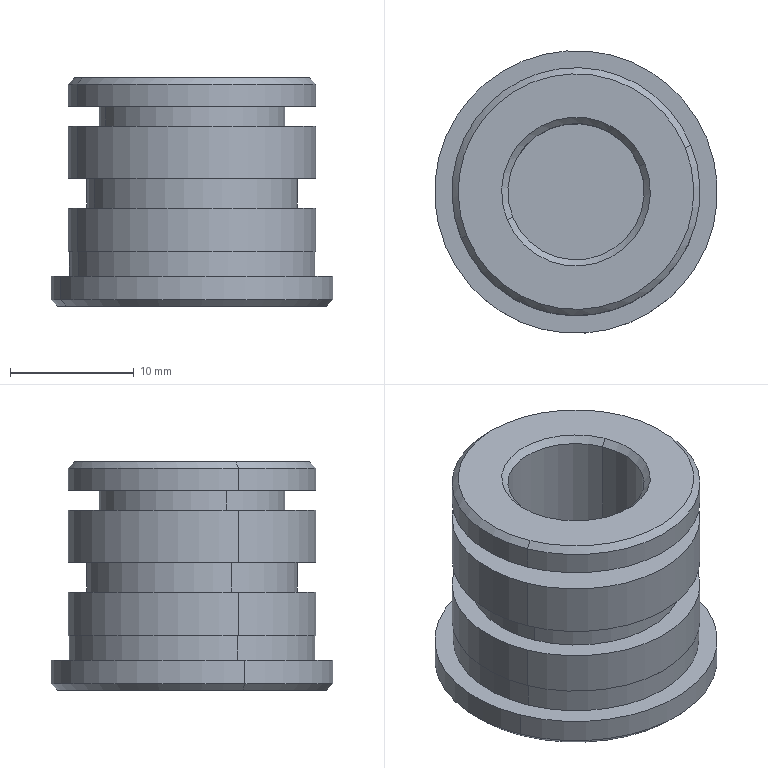Part | SolidWorks | features BaseBody 1 | 1 solid | 34 faces | box 22.8 x 22.8 x 18.4 mm | volume 3781 mm3 | cylinder 18 | plane 10 | cone 6 | commonest cylinder face diameters 20 x6 15 x4 11 x2 17 x2 19.8 x2 22.8 x2
STEP:
#1=CARTESIAN_POINT('',(372.994,98.417,-49.5));
#2=VERTEX_POINT('',#1);
#3=CARTESIAN_POINT('',(393.206,106.583,-49.5));
#4=VERTEX_POINT('',#3);
#5=CARTESIAN_POINT('',(383.1,102.5,-49.5));
#6=DIRECTION('',(0.,0.,1.));
#7=DIRECTION('',(-0.9272,-0.3746,0.));
#8=AXIS2_PLACEMENT_3D('',#5,#6,#7);
#9=CIRCLE('',#8,10.9);
#10=EDGE_CURVE('',#2,#4,#9,.T.);
#11=ORIENTED_EDGE('',*,*,#10,.T.);
#12=CARTESIAN_POINT('',(393.67,106.77,-49.));
#13=VERTEX_POINT('',#12);
#14=CARTESIAN_POINT('',(393.67,106.77,-49.));
#15=DIRECTION('',(0.6556,0.2649,0.7071));
#16=VECTOR('',#15,1000.);
#17=LINE('',#14,#16);
#18=EDGE_CURVE('',#4,#13,#17,.T.);
#19=ORIENTED_EDGE('',*,*,#18,.T.);
#20=CARTESIAN_POINT('',(372.53,98.23,-49.));
#21=VERTEX_POINT('',#20);
#22=CARTESIAN_POINT('',(383.1,102.5,-49.));
#23=DIRECTION('',(0.,0.,1.));
#24=DIRECTION('',(-0.9272,-0.3746,0.));
#25=AXIS2_PLACEMENT_3D('',#22,#23,#24);
#26=CIRCLE('',#25,11.4);
#27=EDGE_CURVE('',#21,#13,#26,.T.);
#28=ORIENTED_EDGE('',*,*,#27,.F.);
#29=CARTESIAN_POINT('',(372.53,98.23,-49.));
#30=DIRECTION('',(-0.6556,-0.2649,0.7071));
#31=VECTOR('',#30,1000.);
#32=LINE('',#29,#31);
#33=EDGE_CURVE('',#2,#21,#32,.T.);
#34=ORIENTED_EDGE('',*,*,#33,.F.);
#35=EDGE_LOOP('',(#11,#19,#28,#34));
#36=FACE_OUTER_BOUND('',#35,.T.);
#37=CARTESIAN_POINT('',(383.1,102.5,-49.));
#38=DIRECTION('',(0.,0.,1.));
#39=DIRECTION('',(-0.9272,-0.3746,0.));
#40=AXIS2_PLACEMENT_3D('',#37,#38,#39);
#41=CONICAL_SURFACE('',#40,11.4,0.7854);
#42=ADVANCED_FACE('',(#36),#41,.T.);
#43=ORIENTED_EDGE('',*,*,#27,.T.);
#44=CARTESIAN_POINT('',(393.67,106.77,-47.1));
#45=VERTEX_POINT('',#44);
#46=CARTESIAN_POINT('',(393.67,106.77,-25.779));
#47=DIRECTION('',(0.,0.,1.));
#48=VECTOR('',#47,1000.);
#49=LINE('',#46,#48);
#50=EDGE_CURVE('',#13,#45,#49,.T.);
#51=ORIENTED_EDGE('',*,*,#50,.T.);
#52=CARTESIAN_POINT('',(372.53,98.23,-47.1));
#53=VERTEX_POINT('',#52);
#54=CARTESIAN_POINT('',(383.1,102.5,-47.1));
#55=DIRECTION('',(0.,0.,1.));
#56=DIRECTION('',(-0.9272,-0.3746,0.));
#57=AXIS2_PLACEMENT_3D('',#54,#55,#56);
#58=CIRCLE('',#57,11.4);
#59=EDGE_CURVE('',#53,#45,#58,.T.);
#60=ORIENTED_EDGE('',*,*,#59,.F.);
#61=CARTESIAN_POINT('',(372.53,98.23,-25.779));
#62=DIRECTION('',(0.,0.,1.));
#63=VECTOR('',#62,1000.);
#64=LINE('',#61,#63);
#65=EDGE_CURVE('',#21,#53,#64,.T.);
#66=ORIENTED_EDGE('',*,*,#65,.F.);
#67=EDGE_LOOP('',(#43,#51,#60,#66));
#68=FACE_OUTER_BOUND('',#67,.T.);
#69=CARTESIAN_POINT('',(383.1,102.5,-25.779));
#70=DIRECTION('',(0.,0.,1.));
#71=DIRECTION('',(-0.9272,-0.3746,0.));
#72=AXIS2_PLACEMENT_3D('',#69,#70,#71);
#73=CYLINDRICAL_SURFACE('',#72,11.4);
#74=ADVANCED_FACE('',(#68),#73,.T.);
#75=CARTESIAN_POINT('',(373.921,98.792,-47.1));
#76=VERTEX_POINT('',#75);
#77=CARTESIAN_POINT('',(392.279,106.208,-47.1));
#78=VERTEX_POINT('',#77);
#79=CARTESIAN_POINT('',(383.1,102.5,-47.1));
#80=DIRECTION('',(0.,0.,1.));
#81=DIRECTION('',(-0.9272,-0.3746,0.));
#82=AXIS2_PLACEMENT_3D('',#79,#80,#81);
#83=CIRCLE('',#82,9.9);
#84=EDGE_CURVE('',#76,#78,#83,.T.);
#85=ORIENTED_EDGE('',*,*,#84,.T.);
#86=CARTESIAN_POINT('',(392.279,106.208,-45.1));
#87=VERTEX_POINT('',#86);
#88=CARTESIAN_POINT('',(392.279,106.208,-25.779));
#89=DIRECTION('',(0.,0.,1.));
#90=VECTOR('',#89,1000.);
#91=LINE('',#88,#90);
#92=EDGE_CURVE('',#78,#87,#91,.T.);
#93=ORIENTED_EDGE('',*,*,#92,.T.);
#94=CARTESIAN_POINT('',(373.921,98.792,-45.1));
#95=VERTEX_POINT('',#94);
#96=CARTESIAN_POINT('',(383.1,102.5,-45.1));
#97=DIRECTION('',(0.,0.,1.));
#98=DIRECTION('',(-0.9272,-0.3746,0.));
#99=AXIS2_PLACEMENT_3D('',#96,#97,#98);
#100=CIRCLE('',#99,9.9);
#101=EDGE_CURVE('',#95,#87,#100,.T.);
#102=ORIENTED_EDGE('',*,*,#101,.F.);
#103=CARTESIAN_POINT('',(373.921,98.792,-25.779));
#104=DIRECTION('',(0.,0.,1.));
#105=VECTOR('',#104,1000.);
#106=LINE('',#103,#105);
#107=EDGE_CURVE('',#76,#95,#106,.T.);
#108=ORIENTED_EDGE('',*,*,#107,.F.);
#109=EDGE_LOOP('',(#85,#93,#102,#108));
#110=FACE_OUTER_BOUND('',#109,.T.);
#111=CARTESIAN_POINT('',(383.1,102.5,-25.779));
#112=DIRECTION('',(0.,0.,1.));
#113=DIRECTION('',(-0.9272,-0.3746,0.));
#114=AXIS2_PLACEMENT_3D('',#111,#112,#113);
#115=CYLINDRICAL_SURFACE('',#114,9.9);
#116=ADVANCED_FACE('',(#110),#115,.T.);
#117=CARTESIAN_POINT('',(373.828,98.754,-45.1));
#118=VERTEX_POINT('',#117);
#119=CARTESIAN_POINT('',(392.372,106.246,-45.1));
#120=VERTEX_POINT('',#119);
#121=CARTESIAN_POINT('',(383.1,102.5,-45.1));
#122=DIRECTION('',(0.,0.,1.));
#123=DIRECTION('',(-0.9272,-0.3746,0.));
#124=AXIS2_PLACEMENT_3D('',#121,#122,#123);
#125=CIRCLE('',#124,10.);
#126=EDGE_CURVE('',#118,#120,#125,.T.);
#127=ORIENTED_EDGE('',*,*,#126,.T.);
#128=CARTESIAN_POINT('',(392.372,106.246,-41.6));
#129=VERTEX_POINT('',#128);
#130=CARTESIAN_POINT('',(392.372,106.246,-25.779));
#131=DIRECTION('',(0.,0.,1.));
#132=VECTOR('',#131,1000.);
#133=LINE('',#130,#132);
#134=EDGE_CURVE('',#120,#129,#133,.T.);
#135=ORIENTED_EDGE('',*,*,#134,.T.);
#136=CARTESIAN_POINT('',(373.828,98.754,-41.6));
#137=VERTEX_POINT('',#136);
#138=CARTESIAN_POINT('',(383.1,102.5,-41.6));
#139=DIRECTION('',(0.,0.,1.));
#140=DIRECTION('',(-0.9272,-0.3746,0.));
#141=AXIS2_PLACEMENT_3D('',#138,#139,#140);
#142=CIRCLE('',#141,10.);
#143=EDGE_CURVE('',#137,#129,#142,.T.);
#144=ORIENTED_EDGE('',*,*,#143,.F.);
#145=CARTESIAN_POINT('',(373.828,98.754,-25.779));
#146=DIRECTION('',(0.,0.,1.));
#147=VECTOR('',#146,1000.);
#148=LINE('',#145,#147);
#149=EDGE_CURVE('',#118,#137,#148,.T.);
#150=ORIENTED_EDGE('',*,*,#149,.F.);
#151=EDGE_LOOP('',(#127,#135,#144,#150));
#152=FACE_OUTER_BOUND('',#151,.T.);
#153=CARTESIAN_POINT('',(383.1,102.5,-25.779));
#154=DIRECTION('',(0.,0.,1.));
#155=DIRECTION('',(-0.9272,-0.3746,0.));
#156=AXIS2_PLACEMENT_3D('',#153,#154,#155);
#157=CYLINDRICAL_SURFACE('',#156,10.);
#158=ADVANCED_FACE('',(#152),#157,.T.);
#159=CARTESIAN_POINT('',(375.219,99.316,-41.6));
#160=VERTEX_POINT('',#159);
#161=CARTESIAN_POINT('',(390.981,105.684,-41.6));
#162=VERTEX_POINT('',#161);
#163=CARTESIAN_POINT('',(383.1,102.5,-41.6));
#164=DIRECTION('',(0.,0.,1.));
#165=DIRECTION('',(-0.9272,-0.3746,0.));
#166=AXIS2_PLACEMENT_3D('',#163,#164,#165);
#167=CIRCLE('',#166,8.5);
#168=EDGE_CURVE('',#160,#162,#167,.T.);
#169=ORIENTED_EDGE('',*,*,#168,.T.);
#170=CARTESIAN_POINT('',(390.981,105.684,-39.2));
#171=VERTEX_POINT('',#170);
#172=CARTESIAN_POINT('',(390.981,105.684,-25.779));
#173=DIRECTION('',(0.,0.,1.));
#174=VECTOR('',#173,1000.);
#175=LINE('',#172,#174);
#176=EDGE_CURVE('',#162,#171,#175,.T.);
#177=ORIENTED_EDGE('',*,*,#176,.T.);
#178=CARTESIAN_POINT('',(375.219,99.316,-39.2));
#179=VERTEX_POINT('',#178);
#180=CARTESIAN_POINT('',(383.1,102.5,-39.2));
#181=DIRECTION('',(0.,0.,1.));
#182=DIRECTION('',(-0.9272,-0.3746,0.));
#183=AXIS2_PLACEMENT_3D('',#180,#181,#182);
#184=CIRCLE('',#183,8.5);
#185=EDGE_CURVE('',#179,#171,#184,.T.);
#186=ORIENTED_EDGE('',*,*,#185,.F.);
#187=CARTESIAN_POINT('',(375.219,99.316,-25.779));
#188=DIRECTION('',(0.,0.,1.));
#189=VECTOR('',#188,1000.);
#190=LINE('',#187,#189);
#191=EDGE_CURVE('',#160,#179,#190,.T.);
#192=ORIENTED_EDGE('',*,*,#191,.F.);
#193=EDGE_LOOP('',(#169,#177,#186,#192));
#194=FACE_OUTER_BOUND('',#193,.T.);
#195=CARTESIAN_POINT('',(383.1,102.5,-25.779));
#196=DIRECTION('',(0.,0.,1.));
#197=DIRECTION('',(-0.9272,-0.3746,0.));
#198=AXIS2_PLACEMENT_3D('',#195,#196,#197);
#199=CYLINDRICAL_SURFACE('',#198,8.5);
#200=ADVANCED_FACE('',(#194),#199,.T.);
#201=CARTESIAN_POINT('',(373.828,98.754,-39.2));
#202=VERTEX_POINT('',#201);
#203=CARTESIAN_POINT('',(392.372,106.246,-39.2));
#204=VERTEX_POINT('',#203);
#205=CARTESIAN_POINT('',(383.1,102.5,-39.2));
#206=DIRECTION('',(0.,0.,1.));
#207=DIRECTION('',(-0.9272,-0.3746,0.));
#208=AXIS2_PLACEMENT_3D('',#205,#206,#207);
#209=CIRCLE('',#208,10.);
#210=EDGE_CURVE('',#202,#204,#209,.T.);
#211=ORIENTED_EDGE('',*,*,#210,.T.);
#212=CARTESIAN_POINT('',(392.372,106.246,-35.));
#213=VERTEX_POINT('',#212);
#214=CARTESIAN_POINT('',(392.372,106.246,-25.779));
#215=DIRECTION('',(0.,0.,1.));
#216=VECTOR('',#215,1000.);
#217=LINE('',#214,#216);
#218=EDGE_CURVE('',#204,#213,#217,.T.);
#219=ORIENTED_EDGE('',*,*,#218,.T.);
#220=CARTESIAN_POINT('',(373.828,98.754,-35.));
#221=VERTEX_POINT('',#220);
#222=CARTESIAN_POINT('',(383.1,102.5,-35.));
#223=DIRECTION('',(0.,0.,1.));
#224=DIRECTION('',(-0.9272,-0.3746,0.));
#225=AXIS2_PLACEMENT_3D('',#222,#223,#224);
#226=CIRCLE('',#225,10.);
#227=EDGE_CURVE('',#221,#213,#226,.T.);
#228=ORIENTED_EDGE('',*,*,#227,.F.);
#229=CARTESIAN_POINT('',(373.828,98.754,-25.779));
#230=DIRECTION('',(0.,0.,1.));
#231=VECTOR('',#230,1000.);
#232=LINE('',#229,#231);
#233=EDGE_CURVE('',#202,#221,#232,.T.);
#234=ORIENTED_EDGE('',*,*,#233,.F.);
#235=EDGE_LOOP('',(#211,#219,#228,#234));
#236=FACE_OUTER_BOUND('',#235,.T.);
#237=CARTESIAN_POINT('',(383.1,102.5,-25.779));
#238=DIRECTION('',(0.,0.,1.));
#239=DIRECTION('',(-0.9272,-0.3746,0.));
#240=AXIS2_PLACEMENT_3D('',#237,#238,#239);
#241=CYLINDRICAL_SURFACE('',#240,10.);
#242=ADVANCED_FACE('',(#236),#241,.T.);
#243=CARTESIAN_POINT('',(376.146,99.691,-35.));
#244=VERTEX_POINT('',#243);
#245=CARTESIAN_POINT('',(390.054,105.309,-35.));
#246=VERTEX_POINT('',#245);
#247=CARTESIAN_POINT('',(383.1,102.5,-35.));
#248=DIRECTION('',(0.,0.,1.));
#249=DIRECTION('',(-0.9272,-0.3746,0.));
#250=AXIS2_PLACEMENT_3D('',#247,#248,#249);
#251=CIRCLE('',#250,7.5);
#252=EDGE_CURVE('',#244,#246,#251,.T.);
#253=ORIENTED_EDGE('',*,*,#252,.T.);
#254=CARTESIAN_POINT('',(390.054,105.309,-33.4));
#255=VERTEX_POINT('',#254);
#256=CARTESIAN_POINT('',(390.054,105.309,-25.779));
#257=DIRECTION('',(0.,0.,1.));
#258=VECTOR('',#257,1000.);
#259=LINE('',#256,#258);
#260=EDGE_CURVE('',#246,#255,#259,.T.);
#261=ORIENTED_EDGE('',*,*,#260,.T.);
#262=CARTESIAN_POINT('',(376.146,99.691,-33.4));
#263=VERTEX_POINT('',#262);
#264=CARTESIAN_POINT('',(383.1,102.5,-33.4));
#265=DIRECTION('',(0.,0.,1.));
#266=DIRECTION('',(-0.9272,-0.3746,0.));
#267=AXIS2_PLACEMENT_3D('',#264,#265,#266);
#268=CIRCLE('',#267,7.5);
#269=EDGE_CURVE('',#263,#255,#268,.T.);
#270=ORIENTED_EDGE('',*,*,#269,.F.);
#271=CARTESIAN_POINT('',(376.146,99.691,-25.779));
#272=DIRECTION('',(0.,0.,1.));
#273=VECTOR('',#272,1000.);
#274=LINE('',#271,#273);
#275=EDGE_CURVE('',#244,#263,#274,.T.);
#276=ORIENTED_EDGE('',*,*,#275,.F.);
#277=EDGE_LOOP('',(#253,#261,#270,#276));
#278=FACE_OUTER_BOUND('',#277,.T.);
#279=CARTESIAN_POINT('',(383.1,102.5,-25.779));
#280=DIRECTION('',(0.,0.,1.));
#281=DIRECTION('',(-0.9272,-0.3746,0.));
#282=AXIS2_PLACEMENT_3D('',#279,#280,#281);
#283=CYLINDRICAL_SURFACE('',#282,7.5);
#284=ADVANCED_FACE('',(#278),#283,.T.);
#285=CARTESIAN_POINT('',(373.828,98.754,-33.4));
#286=VERTEX_POINT('',#285);
#287=CARTESIAN_POINT('',(392.372,106.246,-33.4));
#288=VERTEX_POINT('',#287);
#289=CARTESIAN_POINT('',(383.1,102.5,-33.4));
#290=DIRECTION('',(0.,0.,1.));
#291=DIRECTION('',(-0.9272,-0.3746,0.));
#292=AXIS2_PLACEMENT_3D('',#289,#290,#291);
#293=CIRCLE('',#292,10.);
#294=EDGE_CURVE('',#286,#288,#293,.T.);
#295=ORIENTED_EDGE('',*,*,#294,.T.);
#296=CARTESIAN_POINT('',(392.372,106.246,-31.6));
#297=VERTEX_POINT('',#296);
#298=CARTESIAN_POINT('',(392.372,106.246,-25.779));
#299=DIRECTION('',(0.,0.,1.));
#300=VECTOR('',#299,1000.);
#301=LINE('',#298,#300);
#302=EDGE_CURVE('',#288,#297,#301,.T.);
#303=ORIENTED_EDGE('',*,*,#302,.T.);
#304=CARTESIAN_POINT('',(373.828,98.754,-31.6));
#305=VERTEX_POINT('',#304);
#306=CARTESIAN_POINT('',(383.1,102.5,-31.6));
#307=DIRECTION('',(0.,0.,1.));
#308=DIRECTION('',(-0.9272,-0.3746,0.));
#309=AXIS2_PLACEMENT_3D('',#306,#307,#308);
#310=CIRCLE('',#309,10.);
#311=EDGE_CURVE('',#305,#297,#310,.T.);
#312=ORIENTED_EDGE('',*,*,#311,.F.);
#313=CARTESIAN_POINT('',(373.828,98.754,-25.779));
#314=DIRECTION('',(0.,0.,1.));
#315=VECTOR('',#314,1000.);
#316=LINE('',#313,#315);
#317=EDGE_CURVE('',#286,#305,#316,.T.);
#318=ORIENTED_EDGE('',*,*,#317,.F.);
#319=EDGE_LOOP('',(#295,#303,#312,#318));
#320=FACE_OUTER_BOUND('',#319,.T.);
#321=CARTESIAN_POINT('',(383.1,102.5,-25.779));
#322=DIRECTION('',(0.,0.,1.));
#323=DIRECTION('',(-0.9272,-0.3746,0.));
#324=AXIS2_PLACEMENT_3D('',#321,#322,#323);
#325=CYLINDRICAL_SURFACE('',#324,10.);
#326=ADVANCED_FACE('',(#320),#325,.T.);
#327=CARTESIAN_POINT('',(374.292,98.942,-31.1));
#328=VERTEX_POINT('',#327);
#329=CARTESIAN_POINT('',(391.908,106.058,-31.1));
#330=VERTEX_POINT('',#329);
#331=CARTESIAN_POINT('',(383.1,102.5,-31.1));
#332=DIRECTION('',(0.,0.,1.));
#333=DIRECTION('',(-0.9272,-0.3746,0.));
#334=AXIS2_PLACEMENT_3D('',#331,#332,#333);
#335=CIRCLE('',#334,9.5);
#336=EDGE_CURVE('',#328,#330,#335,.T.);
#337=ORIENTED_EDGE('',*,*,#336,.F.);
#338=CARTESIAN_POINT('',(374.292,98.942,-31.1));
#339=DIRECTION('',(-0.6556,-0.2649,-0.7071));
#340=VECTOR('',#339,1000.);
#341=LINE('',#338,#340);
#342=EDGE_CURVE('',#328,#305,#341,.T.);
#343=ORIENTED_EDGE('',*,*,#342,.T.);
#344=ORIENTED_EDGE('',*,*,#311,.T.);
#345=CARTESIAN_POINT('',(391.908,106.058,-31.1));
#346=DIRECTION('',(0.6556,0.2649,-0.7071));
#347=VECTOR('',#346,1000.);
#348=LINE('',#345,#347);
#349=EDGE_CURVE('',#330,#297,#348,.T.);
#350=ORIENTED_EDGE('',*,*,#349,.F.);
#351=EDGE_LOOP('',(#337,#343,#344,#350));
#352=FACE_OUTER_BOUND('',#351,.T.);
#353=CARTESIAN_POINT('',(383.1,102.5,-31.1));
#354=DIRECTION('',(0.,0.,-1.));
#355=DIRECTION('',(0.9272,0.3746,0.));
#356=AXIS2_PLACEMENT_3D('',#353,#354,#355);
#357=CONICAL_SURFACE('',#356,9.5,0.7854);
#358=ADVANCED_FACE('',(#352),#357,.T.);
#359=CARTESIAN_POINT('',(388.2,104.56,-31.6));
#360=VERTEX_POINT('',#359);
#361=CARTESIAN_POINT('',(378.,100.44,-31.6));
#362=VERTEX_POINT('',#361);
#363=CARTESIAN_POINT('',(383.1,102.5,-31.6));
#364=DIRECTION('',(0.,0.,1.));
#365=DIRECTION('',(-0.9272,-0.3746,0.));
#366=AXIS2_PLACEMENT_3D('',#363,#364,#365);
#367=CIRCLE('',#366,5.5);
#368=EDGE_CURVE('',#360,#362,#367,.T.);
#369=ORIENTED_EDGE('',*,*,#368,.F.);
#370=CARTESIAN_POINT('',(388.663,104.747,-31.1));
#371=VERTEX_POINT('',#370);
#372=CARTESIAN_POINT('',(388.2,104.56,-31.6));
#373=DIRECTION('',(0.6556,0.2649,0.7071));
#374=VECTOR('',#373,1000.);
#375=LINE('',#372,#374);
#376=EDGE_CURVE('',#360,#371,#375,.T.);
#377=ORIENTED_EDGE('',*,*,#376,.T.);
#378=CARTESIAN_POINT('',(377.537,100.253,-31.1));
#379=VERTEX_POINT('',#378);
#380=CARTESIAN_POINT('',(383.1,102.5,-31.1));
#381=DIRECTION('',(0.,0.,1.));
#382=DIRECTION('',(-0.9272,-0.3746,0.));
#383=AXIS2_PLACEMENT_3D('',#380,#381,#382);
#384=CIRCLE('',#383,6.);
#385=EDGE_CURVE('',#371,#379,#384,.T.);
#386=ORIENTED_EDGE('',*,*,#385,.T.);
#387=CARTESIAN_POINT('',(378.,100.44,-31.6));
#388=DIRECTION('',(-0.6556,-0.2649,0.7071));
#389=VECTOR('',#388,1000.);
#390=LINE('',#387,#389);
#391=EDGE_CURVE('',#362,#379,#390,.T.);
#392=ORIENTED_EDGE('',*,*,#391,.F.);
#393=EDGE_LOOP('',(#369,#377,#386,#392));
#394=FACE_OUTER_BOUND('',#393,.T.);
#395=CARTESIAN_POINT('',(383.1,102.5,-31.6));
#396=DIRECTION('',(0.,0.,1.));
#397=DIRECTION('',(-0.9272,-0.3746,0.));
#398=AXIS2_PLACEMENT_3D('',#395,#396,#397);
#399=CONICAL_SURFACE('',#398,5.5,0.7854);
#400=ADVANCED_FACE('',(#394),#399,.F.);
#401=CARTESIAN_POINT('',(388.2,104.56,-45.));
#402=VERTEX_POINT('',#401);
#403=CARTESIAN_POINT('',(378.,100.44,-45.));
#404=VERTEX_POINT('',#403);
#405=CARTESIAN_POINT('',(383.1,102.5,-45.));
#406=DIRECTION('',(0.,0.,1.));
#407=DIRECTION('',(-0.9272,-0.3746,0.));
#408=AXIS2_PLACEMENT_3D('',#405,#406,#407);
#409=CIRCLE('',#408,5.5);
#410=EDGE_CURVE('',#402,#404,#409,.T.);
#411=ORIENTED_EDGE('',*,*,#410,.F.);
#412=CARTESIAN_POINT('',(388.2,104.56,-25.779));
#413=DIRECTION('',(0.,0.,1.));
#414=VECTOR('',#413,1000.);
#415=LINE('',#412,#414);
#416=EDGE_CURVE('',#402,#360,#415,.T.);
#417=ORIENTED_EDGE('',*,*,#416,.T.);
#418=ORIENTED_EDGE('',*,*,#368,.T.);
#419=CARTESIAN_POINT('',(378.,100.44,-25.779));
#420=DIRECTION('',(0.,0.,1.));
#421=VECTOR('',#420,1000.);
#422=LINE('',#419,#421);
#423=EDGE_CURVE('',#404,#362,#422,.T.);
#424=ORIENTED_EDGE('',*,*,#423,.F.);
#425=EDGE_LOOP('',(#411,#417,#418,#424));
#426=FACE_OUTER_BOUND('',#425,.T.);
#427=CARTESIAN_POINT('',(383.1,102.5,-25.779));
#428=DIRECTION('',(0.,0.,1.));
#429=DIRECTION('',(-0.9272,-0.3746,0.));
#430=AXIS2_PLACEMENT_3D('',#427,#428,#429);
#431=CYLINDRICAL_SURFACE('',#430,5.5);
#432=ADVANCED_FACE('',(#426),#431,.F.);
#433=CARTESIAN_POINT('',(390.054,105.309,-47.5));
#434=VERTEX_POINT('',#433);
#435=CARTESIAN_POINT('',(376.146,99.691,-47.5));
#436=VERTEX_POINT('',#435);
#437=CARTESIAN_POINT('',(383.1,102.5,-47.5));
#438=DIRECTION('',(0.,0.,1.));
#439=DIRECTION('',(-0.9272,-0.3746,0.));
#440=AXIS2_PLACEMENT_3D('',#437,#438,#439);
#441=CIRCLE('',#440,7.5);
#442=EDGE_CURVE('',#434,#436,#441,.T.);
#443=ORIENTED_EDGE('',*,*,#442,.F.);
#444=CARTESIAN_POINT('',(390.054,105.309,-45.));
#445=VERTEX_POINT('',#444);
#446=CARTESIAN_POINT('',(390.054,105.309,-25.779));
#447=DIRECTION('',(0.,0.,1.));
#448=VECTOR('',#447,1000.);
#449=LINE('',#446,#448);
#450=EDGE_CURVE('',#434,#445,#449,.T.);
#451=ORIENTED_EDGE('',*,*,#450,.T.);
#452=CARTESIAN_POINT('',(376.146,99.691,-45.));
#453=VERTEX_POINT('',#452);
#454=CARTESIAN_POINT('',(383.1,102.5,-45.));
#455=DIRECTION('',(0.,0.,1.));
#456=DIRECTION('',(-0.9272,-0.3746,0.));
#457=AXIS2_PLACEMENT_3D('',#454,#455,#456);
#458=CIRCLE('',#457,7.5);
#459=EDGE_CURVE('',#445,#453,#458,.T.);
#460=ORIENTED_EDGE('',*,*,#459,.T.);
#461=CARTESIAN_POINT('',(376.146,99.691,-25.779));
#462=DIRECTION('',(0.,0.,1.));
#463=VECTOR('',#462,1000.);
#464=LINE('',#461,#463);
#465=EDGE_CURVE('',#436,#453,#464,.T.);
#466=ORIENTED_EDGE('',*,*,#465,.F.);
#467=EDGE_LOOP('',(#443,#451,#460,#466));
#468=FACE_OUTER_BOUND('',#467,.T.);
#469=CARTESIAN_POINT('',(383.1,102.5,-25.779));
#470=DIRECTION('',(0.,0.,1.));
#471=DIRECTION('',(-0.9272,-0.3746,0.));
#472=AXIS2_PLACEMENT_3D('',#469,#470,#471);
#473=CYLINDRICAL_SURFACE('',#472,7.5);
#474=ADVANCED_FACE('',(#468),#473,.F.);
#475=CARTESIAN_POINT('',(383.1,102.5,-47.5));
#476=DIRECTION('',(0.,0.,1.));
#477=DIRECTION('',(-0.9272,-0.3746,0.));
#478=AXIS2_PLACEMENT_3D('',#475,#476,#477);
#479=CIRCLE('',#478,7.5);
#480=EDGE_CURVE('',#436,#434,#479,.T.);
#481=ORIENTED_EDGE('',*,*,#480,.T.);
#482=ORIENTED_EDGE('',*,*,#442,.T.);
#483=EDGE_LOOP('',(#481,#482));
#484=FACE_OUTER_BOUND('',#483,.T.);
#485=CARTESIAN_POINT('',(383.1,102.5,-47.5));
#486=DIRECTION('',(0.,0.,1.));
#487=DIRECTION('',(-0.9272,-0.3746,0.));
#488=AXIS2_PLACEMENT_3D('',#485,#486,#487);
#489=PLANE('',#488);
#490=ADVANCED_FACE('',(#484),#489,.T.);
#491=ORIENTED_EDGE('',*,*,#450,.F.);
#492=ORIENTED_EDGE('',*,*,#480,.F.);
#493=ORIENTED_EDGE('',*,*,#465,.T.);
#494=CARTESIAN_POINT('',(383.1,102.5,-45.));
#495=DIRECTION('',(0.,0.,1.));
#496=DIRECTION('',(-0.9272,-0.3746,0.));
#497=AXIS2_PLACEMENT_3D('',#494,#495,#496);
#498=CIRCLE('',#497,7.5);
#499=EDGE_CURVE('',#453,#445,#498,.T.);
#500=ORIENTED_EDGE('',*,*,#499,.T.);
#501=EDGE_LOOP('',(#491,#492,#493,#500));
#502=FACE_OUTER_BOUND('',#501,.T.);
#503=CARTESIAN_POINT('',(383.1,102.5,-25.779));
#504=DIRECTION('',(0.,0.,1.));
#505=DIRECTION('',(-0.9272,-0.3746,0.));
#506=AXIS2_PLACEMENT_3D('',#503,#504,#505);
#507=CYLINDRICAL_SURFACE('',#506,7.5);
#508=ADVANCED_FACE('',(#502),#507,.F.);
#509=CARTESIAN_POINT('',(383.1,102.5,-45.));
#510=DIRECTION('',(0.,0.,1.));
#511=DIRECTION('',(-0.9272,-0.3746,0.));
#512=AXIS2_PLACEMENT_3D('',#509,#510,#511);
#513=CIRCLE('',#512,5.5);
#514=EDGE_CURVE('',#404,#402,#513,.T.);
#515=ORIENTED_EDGE('',*,*,#514,.T.);
#516=ORIENTED_EDGE('',*,*,#410,.T.);
#517=EDGE_LOOP('',(#515,#516));
#518=FACE_BOUND('',#517,.T.);
#519=ORIENTED_EDGE('',*,*,#499,.F.);
#520=ORIENTED_EDGE('',*,*,#459,.F.);
#521=EDGE_LOOP('',(#519,#520));
#522=FACE_OUTER_BOUND('',#521,.T.);
#523=CARTESIAN_POINT('',(385.16,97.4,-45.));
#524=DIRECTION('',(0.,0.,-1.));
#525=DIRECTION('',(0.9272,0.3746,0.));
#526=AXIS2_PLACEMENT_3D('',#523,#524,#525);
#527=PLANE('',#526);
#528=ADVANCED_FACE('',(#518,#522),#527,.T.);
#529=ORIENTED_EDGE('',*,*,#416,.F.);
#530=ORIENTED_EDGE('',*,*,#514,.F.);
#531=ORIENTED_EDGE('',*,*,#423,.T.);
#532=CARTESIAN_POINT('',(383.1,102.5,-31.6));
#533=DIRECTION('',(0.,0.,1.));
#534=DIRECTION('',(-0.9272,-0.3746,0.));
#535=AXIS2_PLACEMENT_3D('',#532,#533,#534);
#536=CIRCLE('',#535,5.5);
#537=EDGE_CURVE('',#362,#360,#536,.T.);
#538=ORIENTED_EDGE('',*,*,#537,.T.);
#539=EDGE_LOOP('',(#529,#530,#531,#538));
#540=FACE_OUTER_BOUND('',#539,.T.);
#541=CARTESIAN_POINT('',(383.1,102.5,-25.779));
#542=DIRECTION('',(0.,0.,1.));
#543=DIRECTION('',(-0.9272,-0.3746,0.));
#544=AXIS2_PLACEMENT_3D('',#541,#542,#543);
#545=CYLINDRICAL_SURFACE('',#544,5.5);
#546=ADVANCED_FACE('',(#540),#545,.F.);
#547=ORIENTED_EDGE('',*,*,#376,.F.);
#548=ORIENTED_EDGE('',*,*,#537,.F.);
#549=ORIENTED_EDGE('',*,*,#391,.T.);
#550=CARTESIAN_POINT('',(383.1,102.5,-31.1));
#551=DIRECTION('',(0.,0.,1.));
#552=DIRECTION('',(-0.9272,-0.3746,0.));
#553=AXIS2_PLACEMENT_3D('',#550,#551,#552);
#554=CIRCLE('',#553,6.);
#555=EDGE_CURVE('',#379,#371,#554,.T.);
#556=ORIENTED_EDGE('',*,*,#555,.T.);
#557=EDGE_LOOP('',(#547,#548,#549,#556));
#558=FACE_OUTER_BOUND('',#557,.T.);
#559=CARTESIAN_POINT('',(383.1,102.5,-31.6));
#560=DIRECTION('',(0.,0.,1.));
#561=DIRECTION('',(-0.9272,-0.3746,0.));
#562=AXIS2_PLACEMENT_3D('',#559,#560,#561);
#563=CONICAL_SURFACE('',#562,5.5,0.7854);
#564=ADVANCED_FACE('',(#558),#563,.F.);
#565=CARTESIAN_POINT('',(383.1,102.5,-31.1));
#566=DIRECTION('',(0.,0.,1.));
#567=DIRECTION('',(-0.9272,-0.3746,0.));
#568=AXIS2_PLACEMENT_3D('',#565,#566,#567);
#569=CIRCLE('',#568,9.5);
#570=EDGE_CURVE('',#330,#328,#569,.T.);
#571=ORIENTED_EDGE('',*,*,#570,.T.);
#572=ORIENTED_EDGE('',*,*,#336,.T.);
#573=EDGE_LOOP('',(#571,#572));
#574=FACE_OUTER_BOUND('',#573,.T.);
#575=ORIENTED_EDGE('',*,*,#555,.F.);
#576=ORIENTED_EDGE('',*,*,#385,.F.);
#577=EDGE_LOOP('',(#575,#576));
#578=FACE_BOUND('',#577,.T.);
#579=CARTESIAN_POINT('',(385.347,96.937,-31.1));
#580=DIRECTION('',(0.,0.,1.));
#581=DIRECTION('',(-0.9272,-0.3746,0.));
#582=AXIS2_PLACEMENT_3D('',#579,#580,#581);
#583=PLANE('',#582);
#584=ADVANCED_FACE('',(#574,#578),#583,.T.);
#585=ORIENTED_EDGE('',*,*,#342,.F.);
#586=ORIENTED_EDGE('',*,*,#570,.F.);
#587=ORIENTED_EDGE('',*,*,#349,.T.);
#588=CARTESIAN_POINT('',(383.1,102.5,-31.6));
#589=DIRECTION('',(0.,0.,1.));
#590=DIRECTION('',(-0.9272,-0.3746,0.));
#591=AXIS2_PLACEMENT_3D('',#588,#589,#590);
#592=CIRCLE('',#591,10.);
#593=EDGE_CURVE('',#297,#305,#592,.T.);
#594=ORIENTED_EDGE('',*,*,#593,.T.);
#595=EDGE_LOOP('',(#585,#586,#587,#594));
#596=FACE_OUTER_BOUND('',#595,.T.);
#597=CARTESIAN_POINT('',(383.1,102.5,-31.1));
#598=DIRECTION('',(0.,0.,-1.));
#599=DIRECTION('',(0.9272,0.3746,0.));
#600=AXIS2_PLACEMENT_3D('',#597,#598,#599);
#601=CONICAL_SURFACE('',#600,9.5,0.7854);
#602=ADVANCED_FACE('',(#596),#601,.T.);
#603=ORIENTED_EDGE('',*,*,#302,.F.);
#604=CARTESIAN_POINT('',(383.1,102.5,-33.4));
#605=DIRECTION('',(0.,0.,1.));
#606=DIRECTION('',(-0.9272,-0.3746,0.));
#607=AXIS2_PLACEMENT_3D('',#604,#605,#606);
#608=CIRCLE('',#607,10.);
#609=EDGE_CURVE('',#288,#286,#608,.T.);
#610=ORIENTED_EDGE('',*,*,#609,.T.);
#611=ORIENTED_EDGE('',*,*,#317,.T.);
#612=ORIENTED_EDGE('',*,*,#593,.F.);
#613=EDGE_LOOP('',(#603,#610,#611,#612));
#614=FACE_OUTER_BOUND('',#613,.T.);
#615=CARTESIAN_POINT('',(383.1,102.5,-25.779));
#616=DIRECTION('',(0.,0.,1.));
#617=DIRECTION('',(-0.9272,-0.3746,0.));
#618=AXIS2_PLACEMENT_3D('',#615,#616,#617);
#619=CYLINDRICAL_SURFACE('',#618,10.);
#620=ADVANCED_FACE('',(#614),#619,.T.);
#621=ORIENTED_EDGE('',*,*,#269,.T.);
#622=CARTESIAN_POINT('',(383.1,102.5,-33.4));
#623=DIRECTION('',(0.,0.,1.));
#624=DIRECTION('',(-0.9272,-0.3746,0.));
#625=AXIS2_PLACEMENT_3D('',#622,#623,#624);
#626=CIRCLE('',#625,7.5);
#627=EDGE_CURVE('',#255,#263,#626,.T.);
#628=ORIENTED_EDGE('',*,*,#627,.T.);
#629=EDGE_LOOP('',(#621,#628));
#630=FACE_BOUND('',#629,.T.);
#631=ORIENTED_EDGE('',*,*,#294,.F.);
#632=ORIENTED_EDGE('',*,*,#609,.F.);
#633=EDGE_LOOP('',(#631,#632));
#634=FACE_OUTER_BOUND('',#633,.T.);
#635=CARTESIAN_POINT('',(385.909,95.546,-33.4));
#636=DIRECTION('',(0.,0.,-1.));
#637=DIRECTION('',(0.9272,0.3746,0.));
#638=AXIS2_PLACEMENT_3D('',#635,#636,#637);
#639=PLANE('',#638);
#640=ADVANCED_FACE('',(#630,#634),#639,.T.);
#641=ORIENTED_EDGE('',*,*,#260,.F.);
#642=CARTESIAN_POINT('',(383.1,102.5,-35.));
#643=DIRECTION('',(0.,0.,1.));
#644=DIRECTION('',(-0.9272,-0.3746,0.));
#645=AXIS2_PLACEMENT_3D('',#642,#643,#644);
#646=CIRCLE('',#645,7.5);
#647=EDGE_CURVE('',#246,#244,#646,.T.);
#648=ORIENTED_EDGE('',*,*,#647,.T.);
#649=ORIENTED_EDGE('',*,*,#275,.T.);
#650=ORIENTED_EDGE('',*,*,#627,.F.);
#651=EDGE_LOOP('',(#641,#648,#649,#650));
#652=FACE_OUTER_BOUND('',#651,.T.);
#653=CARTESIAN_POINT('',(383.1,102.5,-25.779));
#654=DIRECTION('',(0.,0.,1.));
#655=DIRECTION('',(-0.9272,-0.3746,0.));
#656=AXIS2_PLACEMENT_3D('',#653,#654,#655);
#657=CYLINDRICAL_SURFACE('',#656,7.5);
#658=ADVANCED_FACE('',(#652),#657,.T.);
#659=ORIENTED_EDGE('',*,*,#227,.T.);
#660=CARTESIAN_POINT('',(383.1,102.5,-35.));
#661=DIRECTION('',(0.,0.,1.));
#662=DIRECTION('',(-0.9272,-0.3746,0.));
#663=AXIS2_PLACEMENT_3D('',#660,#661,#662);
#664=CIRCLE('',#663,10.);
#665=EDGE_CURVE('',#213,#221,#664,.T.);
#666=ORIENTED_EDGE('',*,*,#665,.T.);
#667=EDGE_LOOP('',(#659,#666));
#668=FACE_OUTER_BOUND('',#667,.T.);
#669=ORIENTED_EDGE('',*,*,#252,.F.);
#670=ORIENTED_EDGE('',*,*,#647,.F.);
#671=EDGE_LOOP('',(#669,#670));
#672=FACE_BOUND('',#671,.T.);
#673=CARTESIAN_POINT('',(385.909,95.546,-35.));
#674=DIRECTION('',(0.,0.,1.));
#675=DIRECTION('',(-0.9272,-0.3746,0.));
#676=AXIS2_PLACEMENT_3D('',#673,#674,#675);
#677=PLANE('',#676);
#678=ADVANCED_FACE('',(#668,#672),#677,.T.);
#679=ORIENTED_EDGE('',*,*,#218,.F.);
#680=CARTESIAN_POINT('',(383.1,102.5,-39.2));
#681=DIRECTION('',(0.,0.,1.));
#682=DIRECTION('',(-0.9272,-0.3746,0.));
#683=AXIS2_PLACEMENT_3D('',#680,#681,#682);
#684=CIRCLE('',#683,10.);
#685=EDGE_CURVE('',#204,#202,#684,.T.);
#686=ORIENTED_EDGE('',*,*,#685,.T.);
#687=ORIENTED_EDGE('',*,*,#233,.T.);
#688=ORIENTED_EDGE('',*,*,#665,.F.);
#689=EDGE_LOOP('',(#679,#686,#687,#688));
#690=FACE_OUTER_BOUND('',#689,.T.);
#691=CARTESIAN_POINT('',(383.1,102.5,-25.779));
#692=DIRECTION('',(0.,0.,1.));
#693=DIRECTION('',(-0.9272,-0.3746,0.));
#694=AXIS2_PLACEMENT_3D('',#691,#692,#693);
#695=CYLINDRICAL_SURFACE('',#694,10.);
#696=ADVANCED_FACE('',(#690),#695,.T.);
#697=ORIENTED_EDGE('',*,*,#185,.T.);
#698=CARTESIAN_POINT('',(383.1,102.5,-39.2));
#699=DIRECTION('',(0.,0.,1.));
#700=DIRECTION('',(-0.9272,-0.3746,0.));
#701=AXIS2_PLACEMENT_3D('',#698,#699,#700);
#702=CIRCLE('',#701,8.5);
#703=EDGE_CURVE('',#171,#179,#702,.T.);
#704=ORIENTED_EDGE('',*,*,#703,.T.);
#705=EDGE_LOOP('',(#697,#704));
#706=FACE_BOUND('',#705,.T.);
#707=ORIENTED_EDGE('',*,*,#210,.F.);
#708=ORIENTED_EDGE('',*,*,#685,.F.);
#709=EDGE_LOOP('',(#707,#708));
#710=FACE_OUTER_BOUND('',#709,.T.);
#711=CARTESIAN_POINT('',(386.284,94.619,-39.2));
#712=DIRECTION('',(0.,0.,-1.));
#713=DIRECTION('',(0.9272,0.3746,0.));
#714=AXIS2_PLACEMENT_3D('',#711,#712,#713);
#715=PLANE('',#714);
#716=ADVANCED_FACE('',(#706,#710),#715,.T.);
#717=ORIENTED_EDGE('',*,*,#176,.F.);
#718=CARTESIAN_POINT('',(383.1,102.5,-41.6));
#719=DIRECTION('',(0.,0.,1.));
#720=DIRECTION('',(-0.9272,-0.3746,0.));
#721=AXIS2_PLACEMENT_3D('',#718,#719,#720);
#722=CIRCLE('',#721,8.5);
#723=EDGE_CURVE('',#162,#160,#722,.T.);
#724=ORIENTED_EDGE('',*,*,#723,.T.);
#725=ORIENTED_EDGE('',*,*,#191,.T.);
#726=ORIENTED_EDGE('',*,*,#703,.F.);
#727=EDGE_LOOP('',(#717,#724,#725,#726));
#728=FACE_OUTER_BOUND('',#727,.T.);
#729=CARTESIAN_POINT('',(383.1,102.5,-25.779));
#730=DIRECTION('',(0.,0.,1.));
#731=DIRECTION('',(-0.9272,-0.3746,0.));
#732=AXIS2_PLACEMENT_3D('',#729,#730,#731);
#733=CYLINDRICAL_SURFACE('',#732,8.5);
#734=ADVANCED_FACE('',(#728),#733,.T.);
#735=ORIENTED_EDGE('',*,*,#143,.T.);
#736=CARTESIAN_POINT('',(383.1,102.5,-41.6));
#737=DIRECTION('',(0.,0.,1.));
#738=DIRECTION('',(-0.9272,-0.3746,0.));
#739=AXIS2_PLACEMENT_3D('',#736,#737,#738);
#740=CIRCLE('',#739,10.);
#741=EDGE_CURVE('',#129,#137,#740,.T.);
#742=ORIENTED_EDGE('',*,*,#741,.T.);
#743=EDGE_LOOP('',(#735,#742));
#744=FACE_OUTER_BOUND('',#743,.T.);
#745=ORIENTED_EDGE('',*,*,#168,.F.);
#746=ORIENTED_EDGE('',*,*,#723,.F.);
#747=EDGE_LOOP('',(#745,#746));
#748=FACE_BOUND('',#747,.T.);
#749=CARTESIAN_POINT('',(386.284,94.619,-41.6));
#750=DIRECTION('',(0.,0.,1.));
#751=DIRECTION('',(-0.9272,-0.3746,0.));
#752=AXIS2_PLACEMENT_3D('',#749,#750,#751);
#753=PLANE('',#752);
#754=ADVANCED_FACE('',(#744,#748),#753,.T.);
#755=ORIENTED_EDGE('',*,*,#134,.F.);
#756=CARTESIAN_POINT('',(383.1,102.5,-45.1));
#757=DIRECTION('',(0.,0.,1.));
#758=DIRECTION('',(-0.9272,-0.3746,0.));
#759=AXIS2_PLACEMENT_3D('',#756,#757,#758);
#760=CIRCLE('',#759,10.);
#761=EDGE_CURVE('',#120,#118,#760,.T.);
#762=ORIENTED_EDGE('',*,*,#761,.T.);
#763=ORIENTED_EDGE('',*,*,#149,.T.);
#764=ORIENTED_EDGE('',*,*,#741,.F.);
#765=EDGE_LOOP('',(#755,#762,#763,#764));
#766=FACE_OUTER_BOUND('',#765,.T.);
#767=CARTESIAN_POINT('',(383.1,102.5,-25.779));
#768=DIRECTION('',(0.,0.,1.));
#769=DIRECTION('',(-0.9272,-0.3746,0.));
#770=AXIS2_PLACEMENT_3D('',#767,#768,#769);
#771=CYLINDRICAL_SURFACE('',#770,10.);
#772=ADVANCED_FACE('',(#766),#771,.T.);
#773=ORIENTED_EDGE('',*,*,#101,.T.);
#774=CARTESIAN_POINT('',(383.1,102.5,-45.1));
#775=DIRECTION('',(0.,0.,1.));
#776=DIRECTION('',(-0.9272,-0.3746,0.));
#777=AXIS2_PLACEMENT_3D('',#774,#775,#776);
#778=CIRCLE('',#777,9.9);
#779=EDGE_CURVE('',#87,#95,#778,.T.);
#780=ORIENTED_EDGE('',*,*,#779,.T.);
#781=EDGE_LOOP('',(#773,#780));
#782=FACE_BOUND('',#781,.T.);
#783=ORIENTED_EDGE('',*,*,#126,.F.);
#784=ORIENTED_EDGE('',*,*,#761,.F.);
#785=EDGE_LOOP('',(#783,#784));
#786=FACE_OUTER_BOUND('',#785,.T.);
#787=CARTESIAN_POINT('',(386.808,93.321,-45.1));
#788=DIRECTION('',(0.,0.,-1.));
#789=DIRECTION('',(0.9272,0.3746,0.));
#790=AXIS2_PLACEMENT_3D('',#787,#788,#789);
#791=PLANE('',#790);
#792=ADVANCED_FACE('',(#782,#786),#791,.T.);
#793=ORIENTED_EDGE('',*,*,#92,.F.);
#794=CARTESIAN_POINT('',(383.1,102.5,-47.1));
#795=DIRECTION('',(0.,0.,1.));
#796=DIRECTION('',(-0.9272,-0.3746,0.));
#797=AXIS2_PLACEMENT_3D('',#794,#795,#796);
#798=CIRCLE('',#797,9.9);
#799=EDGE_CURVE('',#78,#76,#798,.T.);
#800=ORIENTED_EDGE('',*,*,#799,.T.);
#801=ORIENTED_EDGE('',*,*,#107,.T.);
#802=ORIENTED_EDGE('',*,*,#779,.F.);
#803=EDGE_LOOP('',(#793,#800,#801,#802));
#804=FACE_OUTER_BOUND('',#803,.T.);
#805=CARTESIAN_POINT('',(383.1,102.5,-25.779));
#806=DIRECTION('',(0.,0.,1.));
#807=DIRECTION('',(-0.9272,-0.3746,0.));
#808=AXIS2_PLACEMENT_3D('',#805,#806,#807);
#809=CYLINDRICAL_SURFACE('',#808,9.9);
#810=ADVANCED_FACE('',(#804),#809,.T.);
#811=ORIENTED_EDGE('',*,*,#59,.T.);
#812=CARTESIAN_POINT('',(383.1,102.5,-47.1));
#813=DIRECTION('',(0.,0.,1.));
#814=DIRECTION('',(-0.9272,-0.3746,0.));
#815=AXIS2_PLACEMENT_3D('',#812,#813,#814);
#816=CIRCLE('',#815,11.4);
#817=EDGE_CURVE('',#45,#53,#816,.T.);
#818=ORIENTED_EDGE('',*,*,#817,.T.);
#819=EDGE_LOOP('',(#811,#818));
#820=FACE_OUTER_BOUND('',#819,.T.);
#821=ORIENTED_EDGE('',*,*,#84,.F.);
#822=ORIENTED_EDGE('',*,*,#799,.F.);
#823=EDGE_LOOP('',(#821,#822));
#824=FACE_BOUND('',#823,.T.);
#825=CARTESIAN_POINT('',(386.808,93.321,-47.1));
#826=DIRECTION('',(0.,0.,1.));
#827=DIRECTION('',(-0.9272,-0.3746,0.));
#828=AXIS2_PLACEMENT_3D('',#825,#826,#827);
#829=PLANE('',#828);
#830=ADVANCED_FACE('',(#820,#824),#829,.T.);
#831=ORIENTED_EDGE('',*,*,#50,.F.);
#832=CARTESIAN_POINT('',(383.1,102.5,-49.));
#833=DIRECTION('',(0.,0.,1.));
#834=DIRECTION('',(-0.9272,-0.3746,0.));
#835=AXIS2_PLACEMENT_3D('',#832,#833,#834);
#836=CIRCLE('',#835,11.4);
#837=EDGE_CURVE('',#13,#21,#836,.T.);
#838=ORIENTED_EDGE('',*,*,#837,.T.);
#839=ORIENTED_EDGE('',*,*,#65,.T.);
#840=ORIENTED_EDGE('',*,*,#817,.F.);
#841=EDGE_LOOP('',(#831,#838,#839,#840));
#842=FACE_OUTER_BOUND('',#841,.T.);
#843=CARTESIAN_POINT('',(383.1,102.5,-25.779));
#844=DIRECTION('',(0.,0.,1.));
#845=DIRECTION('',(-0.9272,-0.3746,0.));
#846=AXIS2_PLACEMENT_3D('',#843,#844,#845);
#847=CYLINDRICAL_SURFACE('',#846,11.4);
#848=ADVANCED_FACE('',(#842),#847,.T.);
#849=ORIENTED_EDGE('',*,*,#18,.F.);
#850=CARTESIAN_POINT('',(383.1,102.5,-49.5));
#851=DIRECTION('',(0.,0.,1.));
#852=DIRECTION('',(-0.9272,-0.3746,0.));
#853=AXIS2_PLACEMENT_3D('',#850,#851,#852);
#854=CIRCLE('',#853,10.9);
#855=EDGE_CURVE('',#4,#2,#854,.T.);
#856=ORIENTED_EDGE('',*,*,#855,.T.);
#857=ORIENTED_EDGE('',*,*,#33,.T.);
#858=ORIENTED_EDGE('',*,*,#837,.F.);
#859=EDGE_LOOP('',(#849,#856,#857,#858));
#860=FACE_OUTER_BOUND('',#859,.T.);
#861=CARTESIAN_POINT('',(383.1,102.5,-49.));
#862=DIRECTION('',(0.,0.,1.));
#863=DIRECTION('',(-0.9272,-0.3746,0.));
#864=AXIS2_PLACEMENT_3D('',#861,#862,#863);
#865=CONICAL_SURFACE('',#864,11.4,0.7854);
#866=ADVANCED_FACE('',(#860),#865,.T.);
#867=ORIENTED_EDGE('',*,*,#10,.F.);
#868=ORIENTED_EDGE('',*,*,#855,.F.);
#869=EDGE_LOOP('',(#867,#868));
#870=FACE_OUTER_BOUND('',#869,.T.);
#871=CARTESIAN_POINT('',(383.1,102.5,-49.5));
#872=DIRECTION('',(0.,0.,-1.));
#873=DIRECTION('',(0.9272,0.3746,0.));
#874=AXIS2_PLACEMENT_3D('',#871,#872,#873);
#875=PLANE('',#874);
#876=ADVANCED_FACE('',(#870),#875,.T.);
#877=CLOSED_SHELL('',(#42,#74,#116,#158,#200,#242,#284,#326,#358,#400,#432,#474,#490,#508,#528,#546,#564,#584,#602,#620,#640,#658,#678,#696,#716,#734,#754,#772,#792,#810,#830,#848,#866,#876));
#878=MANIFOLD_SOLID_BREP('',#877);
#879=CARTESIAN_POINT('',(0.,0.,0.));
#880=DIRECTION('',(0.,0.,1.));
#881=DIRECTION('',(1.,0.,0.));
#882=AXIS2_PLACEMENT_3D('',#879,#880,#881);
#883=(LENGTH_UNIT()NAMED_UNIT(*)SI_UNIT(.MILLI.,.METRE.));
#884=UNCERTAINTY_MEASURE_WITH_UNIT(LENGTH_MEASURE(0.00001),#883,'','');
#885=(NAMED_UNIT(*)PLANE_ANGLE_UNIT()SI_UNIT($,.RADIAN.));
#886=(NAMED_UNIT(*)SI_UNIT($,.STERADIAN.)SOLID_ANGLE_UNIT());
#887=(GEOMETRIC_REPRESENTATION_CONTEXT(3)GLOBAL_UNCERTAINTY_ASSIGNED_CONTEXT((#884))GLOBAL_UNIT_ASSIGNED_CONTEXT((#883,#885,#886))REPRESENTATION_CONTEXT('',''));
#888=ADVANCED_BREP_SHAPE_REPRESENTATION('',(#878,#882),#887);